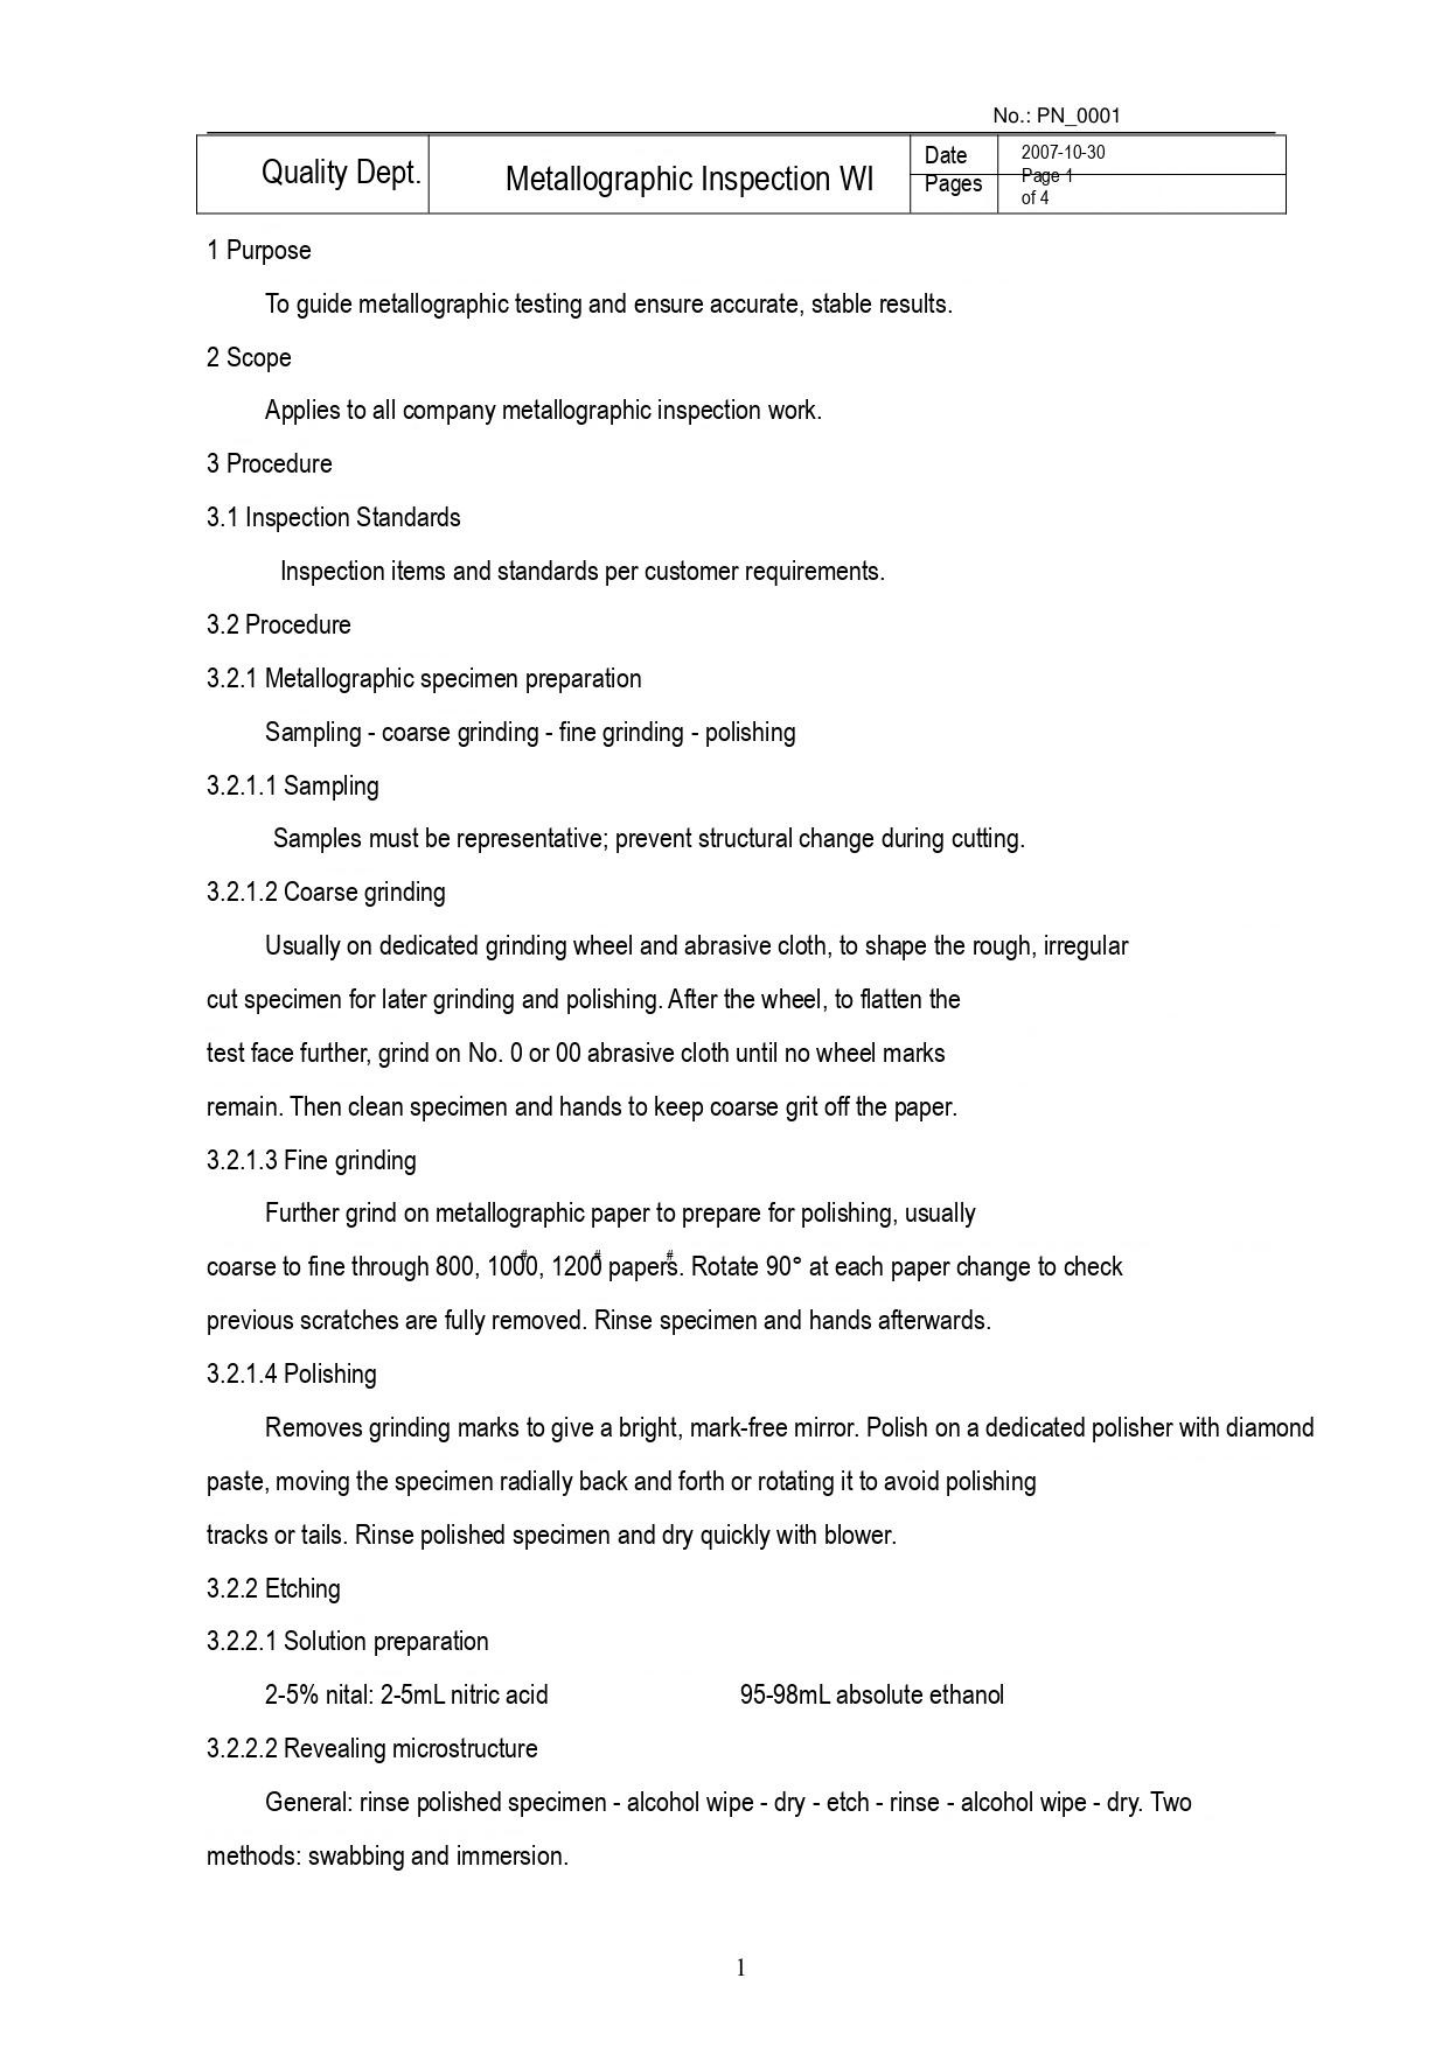No.: PN_0001

| Quality Dept. | Metallographic Inspection WI | Date | 2007-10-30 |
|---|---|---|---|
| | | Pages | Page 1 of 4 |

1 Purpose

To guide metallographic testing and ensure accurate, stable results.

2 Scope

Applies to all company metallographic inspection work.

3 Procedure

3.1 Inspection Standards

Inspection items and standards per customer requirements.

3.2 Procedure

3.2.1 Metallographic specimen preparation

Sampling - coarse grinding - fine grinding - polishing

3.2.1.1 Sampling

Samples must be representative; prevent structural change during cutting.

3.2.1.2 Coarse grinding

Usually on dedicated grinding wheel and abrasive cloth, to shape the rough, irregular cut specimen for later grinding and polishing. After the wheel, to flatten the test face further, grind on No. 0 or 00 abrasive cloth until no wheel marks remain. Then clean specimen and hands to keep coarse grit off the paper.

3.2.1.3 Fine grinding

Further grind on metallographic paper to prepare for polishing, usually coarse to fine through 800, 1000#, 1200# papers. Rotate 90° at each paper change to check previous scratches are fully removed. Rinse specimen and hands afterwards.

3.2.1.4 Polishing

Removes grinding marks to give a bright, mark-free mirror. Polish on a dedicated polisher with diamond paste, moving the specimen radially back and forth or rotating it to avoid polishing tracks or tails. Rinse polished specimen and dry quickly with blower.

3.2.2 Etching

3.2.2.1 Solution preparation

2-5% nital: 2-5mL nitric acid 95-98mL absolute ethanol

3.2.2.2 Revealing microstructure

General: rinse polished specimen - alcohol wipe - dry - etch - rinse - alcohol wipe - dry. Two methods: swabbing and immersion.

1
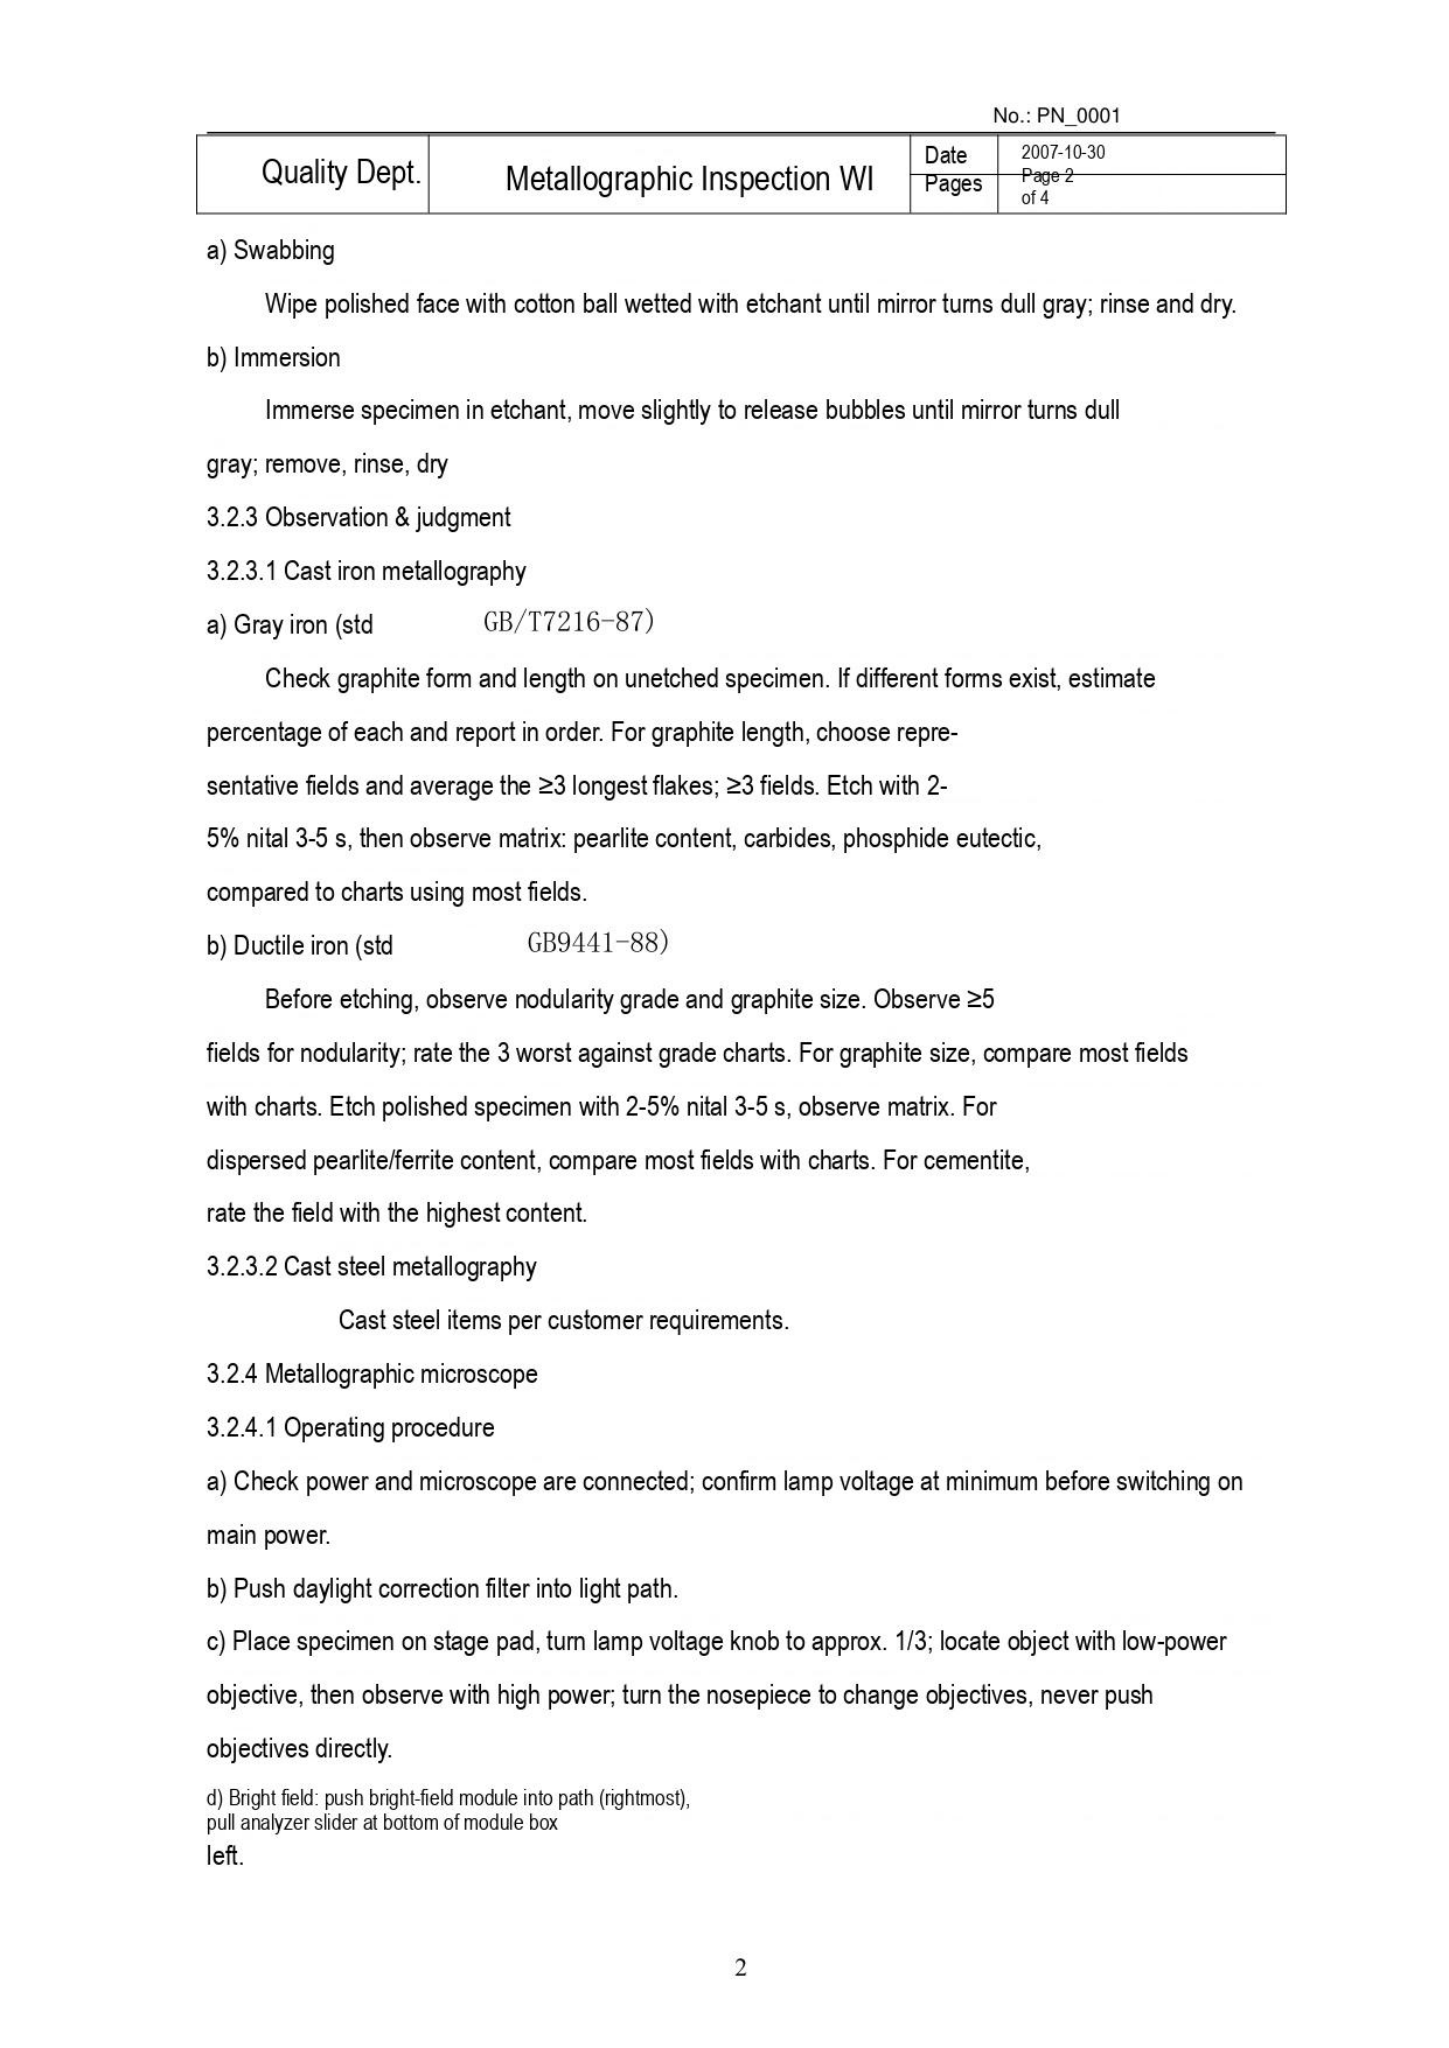No.: PN_0001

| Quality Dept. | Metallographic Inspection WI | Date | 2007-10-30 |
|---|---|---|---|
| | | Pages | Page 2 of 4 |

a) Swabbing

Wipe polished face with cotton ball wetted with etchant until mirror turns dull gray; rinse and dry.

b) Immersion

Immerse specimen in etchant, move slightly to release bubbles until mirror turns dull gray; remove, rinse, dry

3.2.3 Observation & judgment

3.2.3.1 Cast iron metallography

a) Gray iron (std GB/T7216-87)

Check graphite form and length on unetched specimen. If different forms exist, estimate percentage of each and report in order. For graphite length, choose representative fields and average the ≥3 longest flakes; ≥3 fields. Etch with 2-5% nital 3-5 s, then observe matrix: pearlite content, carbides, phosphide eutectic, compared to charts using most fields.

b) Ductile iron (std GB9441-88)

Before etching, observe nodularity grade and graphite size. Observe ≥5 fields for nodularity; rate the 3 worst against grade charts. For graphite size, compare most fields with charts. Etch polished specimen with 2-5% nital 3-5 s, observe matrix. For dispersed pearlite/ferrite content, compare most fields with charts. For cementite, rate the field with the highest content.

3.2.3.2 Cast steel metallography

Cast steel items per customer requirements.

3.2.4 Metallographic microscope

3.2.4.1 Operating procedure

a) Check power and microscope are connected; confirm lamp voltage at minimum before switching on main power.

b) Push daylight correction filter into light path.

c) Place specimen on stage pad, turn lamp voltage knob to approx. 1/3; locate object with low-power objective, then observe with high power; turn the nosepiece to change objectives, never push objectives directly.

d) Bright field: push bright-field module into path (rightmost), pull analyzer slider at bottom of module box left.

2
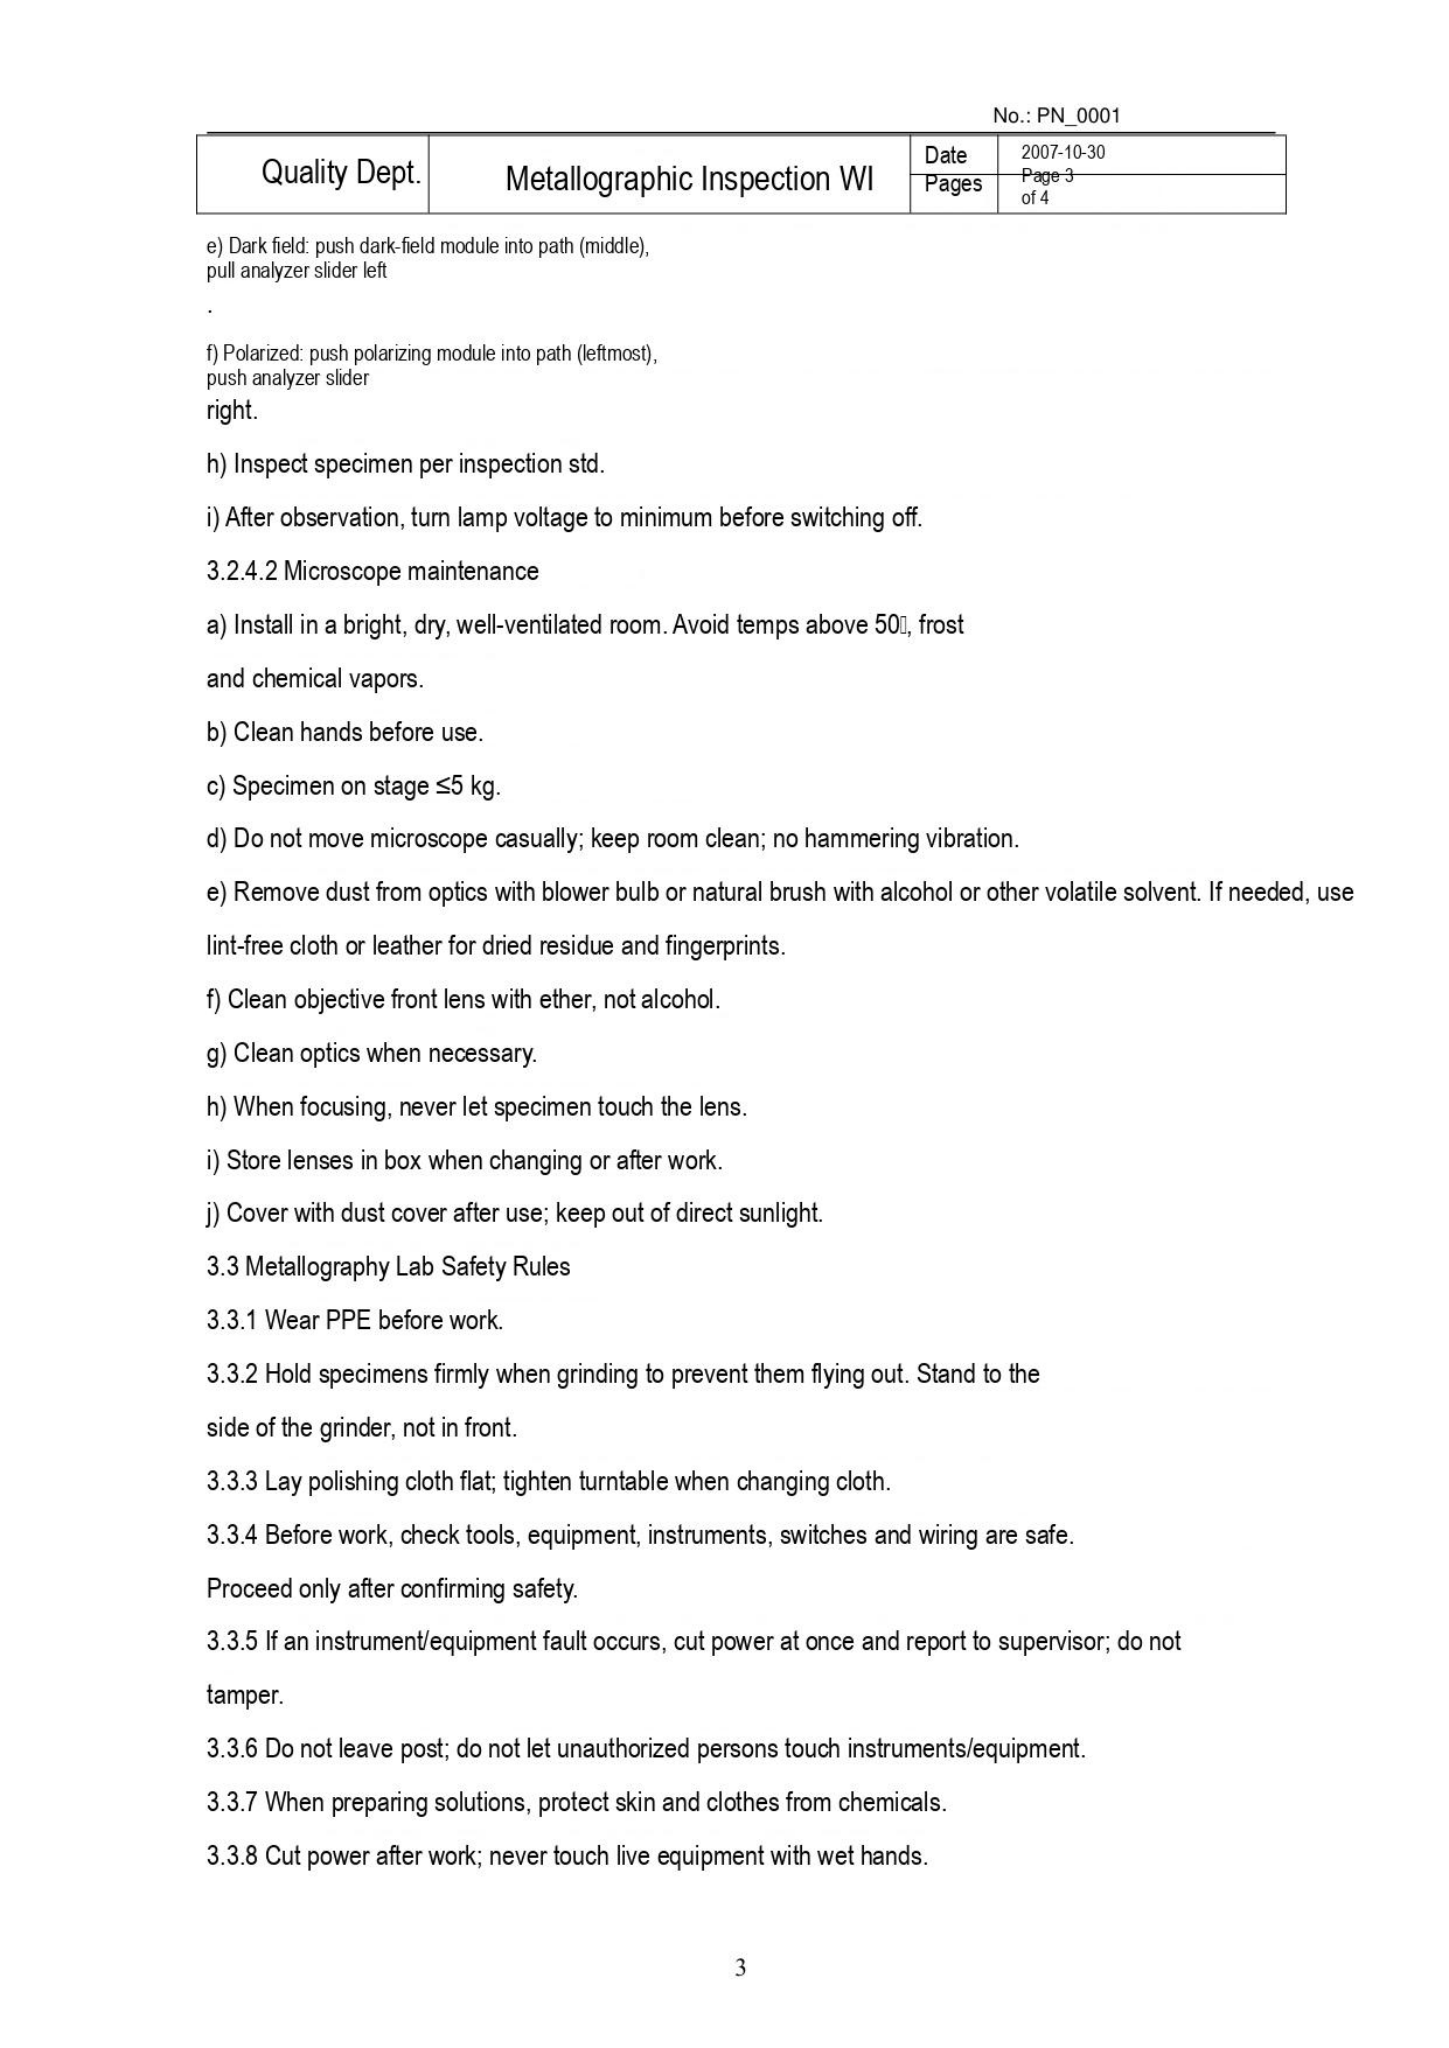No.: PN_0001

| Quality Dept. | Metallographic Inspection WI | Date | 2007-10-30 |
|---|---|---|---|
| | | Pages | Page 3 of 4 |

e) Dark field: push dark-field module into path (middle), pull analyzer slider left

.

f) Polarized: push polarizing module into path (leftmost), push analyzer slider right.

h) Inspect specimen per inspection std.

i) After observation, turn lamp voltage to minimum before switching off.

3.2.4.2 Microscope maintenance

a) Install in a bright, dry, well-ventilated room. Avoid temps above 50, frost and chemical vapors.

b) Clean hands before use.

c) Specimen on stage ≤5 kg.

d) Do not move microscope casually; keep room clean; no hammering vibration.

e) Remove dust from optics with blower bulb or natural brush with alcohol or other volatile solvent. If needed, use lint-free cloth or leather for dried residue and fingerprints.

f) Clean objective front lens with ether, not alcohol.

g) Clean optics when necessary.

h) When focusing, never let specimen touch the lens.

i) Store lenses in box when changing or after work.

j) Cover with dust cover after use; keep out of direct sunlight.

3.3 Metallography Lab Safety Rules

3.3.1 Wear PPE before work.

3.3.2 Hold specimens firmly when grinding to prevent them flying out. Stand to the side of the grinder, not in front.

3.3.3 Lay polishing cloth flat; tighten turntable when changing cloth.

3.3.4 Before work, check tools, equipment, instruments, switches and wiring are safe. Proceed only after confirming safety.

3.3.5 If an instrument/equipment fault occurs, cut power at once and report to supervisor; do not tamper.

3.3.6 Do not leave post; do not let unauthorized persons touch instruments/equipment.

3.3.7 When preparing solutions, protect skin and clothes from chemicals.

3.3.8 Cut power after work; never touch live equipment with wet hands.

3